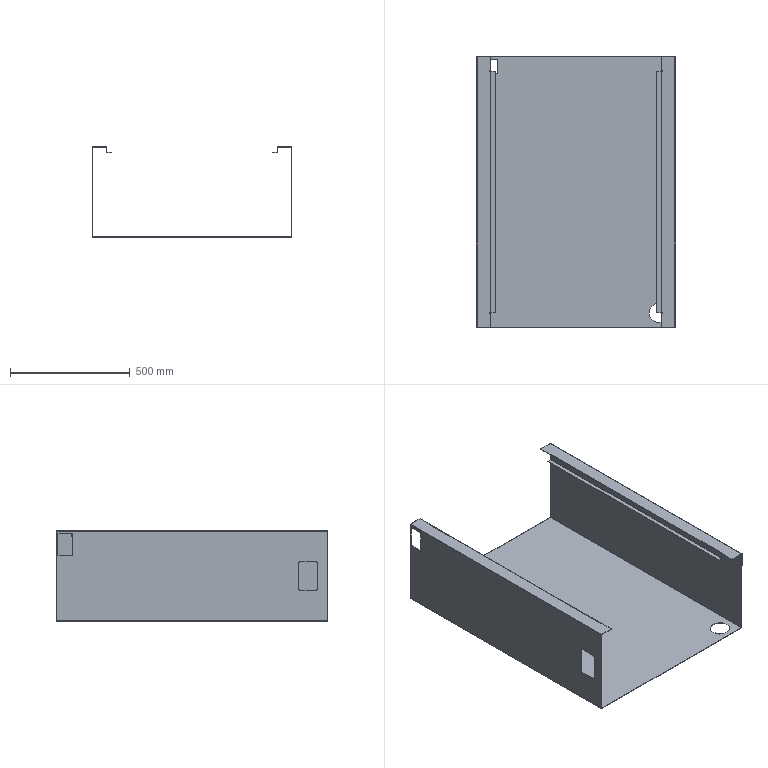Part | STEP file | Electrical Cabinet 1 | 1 solid | 74 faces | box 832 x 1130 x 380 mm | volume 3955545 mm3 | plane 46 | cylinder 28 | commonest cylinder face diameters 1 x14 5 x8 20 x4 80 x2